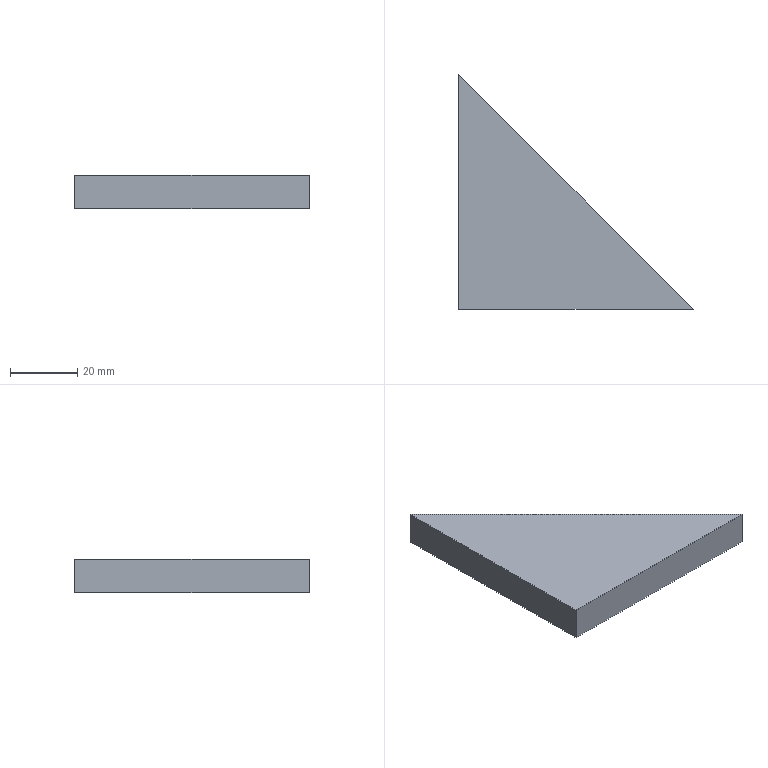Part | SolidWorks | features BaseBody 1 | 1 solid | 5 faces | box 70 x 70 x 10 mm | volume 24500 mm3 | plane 5
STEP:
#1=CARTESIAN_POINT('',(0.,0.,-5.));
#2=VERTEX_POINT('',#1);
#3=CARTESIAN_POINT('',(70.,0.,-5.));
#4=VERTEX_POINT('',#3);
#5=CARTESIAN_POINT('',(0.,0.,-5.));
#6=DIRECTION('',(1.,0.,0.));
#7=VECTOR('',#6,1000.);
#8=LINE('',#5,#7);
#9=EDGE_CURVE('',#2,#4,#8,.T.);
#10=ORIENTED_EDGE('',*,*,#9,.F.);
#11=CARTESIAN_POINT('',(0.,70.,-5.));
#12=VERTEX_POINT('',#11);
#13=CARTESIAN_POINT('',(0.,0.,-5.));
#14=DIRECTION('',(0.,-1.,0.));
#15=VECTOR('',#14,1000.);
#16=LINE('',#13,#15);
#17=EDGE_CURVE('',#12,#2,#16,.T.);
#18=ORIENTED_EDGE('',*,*,#17,.F.);
#19=CARTESIAN_POINT('',(70.,0.,-5.));
#20=DIRECTION('',(-0.7071,0.7071,0.));
#21=VECTOR('',#20,1000.);
#22=LINE('',#19,#21);
#23=EDGE_CURVE('',#4,#12,#22,.T.);
#24=ORIENTED_EDGE('',*,*,#23,.F.);
#25=EDGE_LOOP('',(#10,#18,#24));
#26=FACE_OUTER_BOUND('',#25,.T.);
#27=CARTESIAN_POINT('',(0.,0.,-5.));
#28=DIRECTION('',(0.,0.,1.));
#29=DIRECTION('',(1.,0.,0.));
#30=AXIS2_PLACEMENT_3D('',#27,#28,#29);
#31=PLANE('',#30);
#32=ADVANCED_FACE('',(#26),#31,.F.);
#33=CARTESIAN_POINT('',(0.,70.,5.));
#34=VERTEX_POINT('',#33);
#35=CARTESIAN_POINT('',(0.,70.,5.));
#36=DIRECTION('',(0.,0.,-1.));
#37=VECTOR('',#36,1000.);
#38=LINE('',#35,#37);
#39=EDGE_CURVE('',#34,#12,#38,.T.);
#40=ORIENTED_EDGE('',*,*,#39,.F.);
#41=CARTESIAN_POINT('',(70.,0.,5.));
#42=VERTEX_POINT('',#41);
#43=CARTESIAN_POINT('',(70.,0.,5.));
#44=DIRECTION('',(-0.7071,0.7071,0.));
#45=VECTOR('',#44,1000.);
#46=LINE('',#43,#45);
#47=EDGE_CURVE('',#42,#34,#46,.T.);
#48=ORIENTED_EDGE('',*,*,#47,.F.);
#49=CARTESIAN_POINT('',(70.,0.,5.));
#50=DIRECTION('',(0.,0.,1.));
#51=VECTOR('',#50,1000.);
#52=LINE('',#49,#51);
#53=EDGE_CURVE('',#4,#42,#52,.T.);
#54=ORIENTED_EDGE('',*,*,#53,.F.);
#55=ORIENTED_EDGE('',*,*,#23,.T.);
#56=EDGE_LOOP('',(#40,#48,#54,#55));
#57=FACE_OUTER_BOUND('',#56,.T.);
#58=CARTESIAN_POINT('',(70.,0.,5.));
#59=DIRECTION('',(-0.7071,-0.7071,0.));
#60=DIRECTION('',(0.7071,-0.7071,0.));
#61=AXIS2_PLACEMENT_3D('',#58,#59,#60);
#62=PLANE('',#61);
#63=ADVANCED_FACE('',(#57),#62,.F.);
#64=ORIENTED_EDGE('',*,*,#53,.T.);
#65=CARTESIAN_POINT('',(0.,0.,5.));
#66=VERTEX_POINT('',#65);
#67=CARTESIAN_POINT('',(0.,0.,5.));
#68=DIRECTION('',(1.,0.,0.));
#69=VECTOR('',#68,1000.);
#70=LINE('',#67,#69);
#71=EDGE_CURVE('',#66,#42,#70,.T.);
#72=ORIENTED_EDGE('',*,*,#71,.F.);
#73=CARTESIAN_POINT('',(0.,0.,5.));
#74=DIRECTION('',(0.,0.,1.));
#75=VECTOR('',#74,1000.);
#76=LINE('',#73,#75);
#77=EDGE_CURVE('',#2,#66,#76,.T.);
#78=ORIENTED_EDGE('',*,*,#77,.F.);
#79=ORIENTED_EDGE('',*,*,#9,.T.);
#80=EDGE_LOOP('',(#64,#72,#78,#79));
#81=FACE_OUTER_BOUND('',#80,.T.);
#82=CARTESIAN_POINT('',(0.,0.,5.));
#83=DIRECTION('',(0.,1.,0.));
#84=DIRECTION('',(0.,0.,1.));
#85=AXIS2_PLACEMENT_3D('',#82,#83,#84);
#86=PLANE('',#85);
#87=ADVANCED_FACE('',(#81),#86,.F.);
#88=ORIENTED_EDGE('',*,*,#77,.T.);
#89=CARTESIAN_POINT('',(0.,70.,5.));
#90=DIRECTION('',(0.,-1.,0.));
#91=VECTOR('',#90,1000.);
#92=LINE('',#89,#91);
#93=EDGE_CURVE('',#34,#66,#92,.T.);
#94=ORIENTED_EDGE('',*,*,#93,.F.);
#95=ORIENTED_EDGE('',*,*,#39,.T.);
#96=ORIENTED_EDGE('',*,*,#17,.T.);
#97=EDGE_LOOP('',(#88,#94,#95,#96));
#98=FACE_OUTER_BOUND('',#97,.T.);
#99=CARTESIAN_POINT('',(0.,70.,5.));
#100=DIRECTION('',(1.,0.,0.));
#101=DIRECTION('',(0.,1.,0.));
#102=AXIS2_PLACEMENT_3D('',#99,#100,#101);
#103=PLANE('',#102);
#104=ADVANCED_FACE('',(#98),#103,.F.);
#105=ORIENTED_EDGE('',*,*,#93,.T.);
#106=ORIENTED_EDGE('',*,*,#71,.T.);
#107=ORIENTED_EDGE('',*,*,#47,.T.);
#108=EDGE_LOOP('',(#105,#106,#107));
#109=FACE_OUTER_BOUND('',#108,.T.);
#110=CARTESIAN_POINT('',(0.,0.,5.));
#111=DIRECTION('',(0.,0.,1.));
#112=DIRECTION('',(1.,0.,0.));
#113=AXIS2_PLACEMENT_3D('',#110,#111,#112);
#114=PLANE('',#113);
#115=ADVANCED_FACE('',(#109),#114,.T.);
#116=CLOSED_SHELL('',(#32,#63,#87,#104,#115));
#117=MANIFOLD_SOLID_BREP('',#116);
#118=CARTESIAN_POINT('',(0.,0.,0.));
#119=DIRECTION('',(0.,0.,1.));
#120=DIRECTION('',(1.,0.,0.));
#121=AXIS2_PLACEMENT_3D('',#118,#119,#120);
#122=(LENGTH_UNIT()NAMED_UNIT(*)SI_UNIT(.MILLI.,.METRE.));
#123=UNCERTAINTY_MEASURE_WITH_UNIT(LENGTH_MEASURE(0.00001),#122,'','');
#124=(NAMED_UNIT(*)PLANE_ANGLE_UNIT()SI_UNIT($,.RADIAN.));
#125=(NAMED_UNIT(*)SI_UNIT($,.STERADIAN.)SOLID_ANGLE_UNIT());
#126=(GEOMETRIC_REPRESENTATION_CONTEXT(3)GLOBAL_UNCERTAINTY_ASSIGNED_CONTEXT((#123))GLOBAL_UNIT_ASSIGNED_CONTEXT((#122,#124,#125))REPRESENTATION_CONTEXT('',''));
#127=ADVANCED_BREP_SHAPE_REPRESENTATION('',(#117,#121),#126);